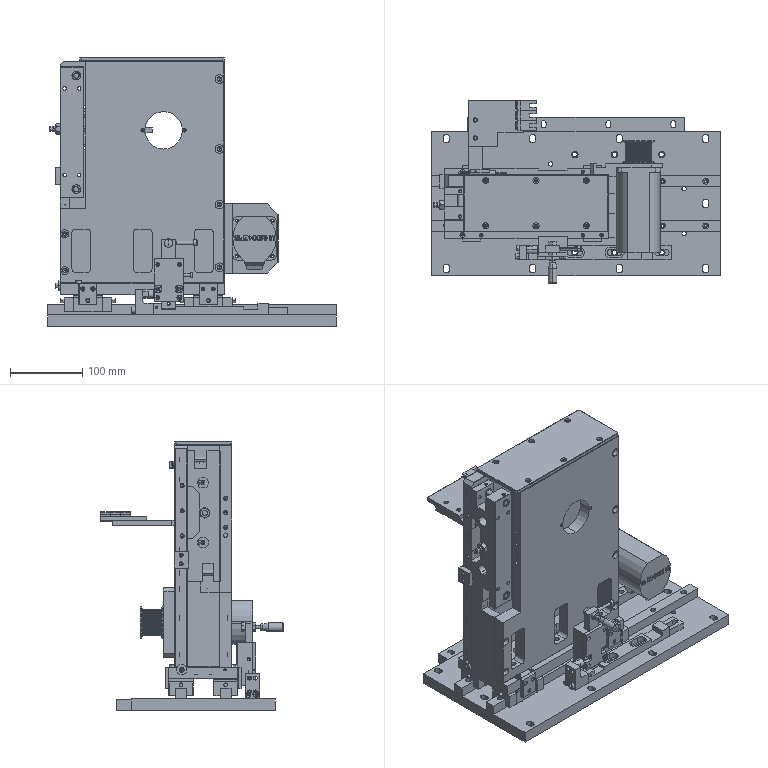Part | NX | 74 solids | 4371 faces | volume 5123702 mm3 | plane 2216 | cylinder 1467 | cone 634 | spline 44 | sphere 6 | torus 4 | commonest cylinder face diameters 5 x413 3.3 x148 4.5 x68 0.5 x52 4.2 x52 6.55 x52